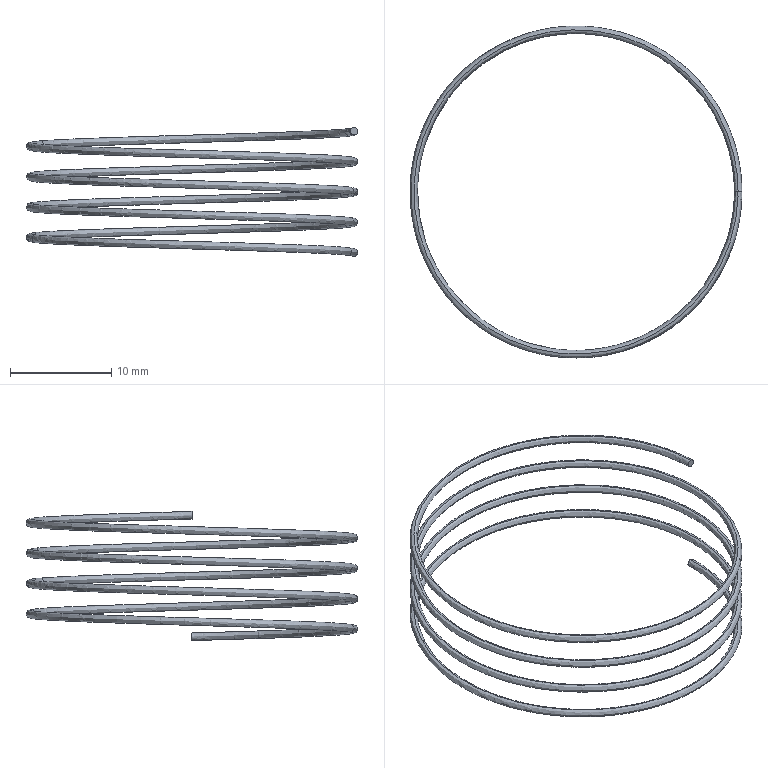Part | STEP file | Return spring | 1 solid | 4 faces | box 32.75 x 32.75 x 12.75 mm | volume 176.657 mm3 | spline 2 | plane 2